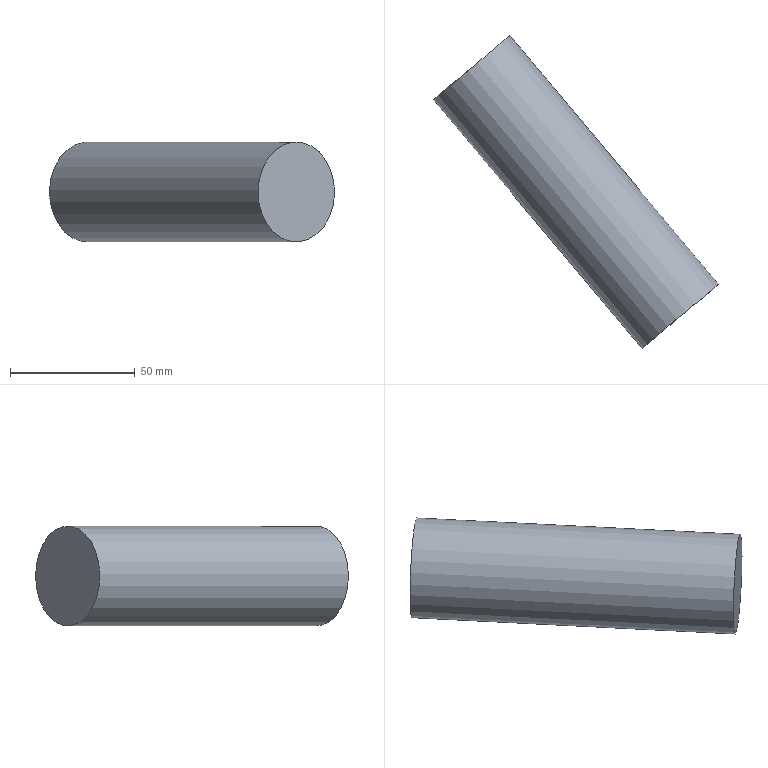Part | NX | features solid 2 | 1 solid | 3 faces | box 114.204 x 125.297 x 40 mm | volume 163363 mm3 | plane 2 | cylinder 1 | commonest cylinder face diameters 40 x1
STEP:
#1=CARTESIAN_POINT('',(828.899,303.057,-194.158));
#2=VERTEX_POINT('',#1);
#3=CARTESIAN_POINT('',(843.885,315.632,-190.));
#4=DIRECTION('',(-0.6428,0.766,0.));
#5=DIRECTION('',(-0.7493,-0.6287,-0.2079));
#6=AXIS2_PLACEMENT_3D('',#3,#4,#5);
#7=CIRCLE('',#6,20.);
#8=EDGE_CURVE('',#2,#2,#7,.F.);
#9=ORIENTED_EDGE('',*,*,#8,.T.);
#10=EDGE_LOOP('',(#9));
#11=FACE_BOUND('',#10,.T.);
#12=CARTESIAN_POINT('',(862.618,331.35,-184.802));
#13=DIRECTION('',(-0.6428,0.766,0.));
#14=DIRECTION('',(0.1593,0.1336,-0.9781));
#15=AXIS2_PLACEMENT_3D('',#12,#13,#14);
#16=PLANE('',#15);
#17=ADVANCED_FACE('',(#11),#16,.F.);
#18=CARTESIAN_POINT('',(745.337,402.643,-194.158));
#19=VERTEX_POINT('',#18);
#20=CARTESIAN_POINT('',(760.323,415.217,-190.));
#21=DIRECTION('',(-0.6428,0.766,0.));
#22=DIRECTION('',(-0.7493,-0.6287,-0.2079));
#23=AXIS2_PLACEMENT_3D('',#20,#21,#22);
#24=CIRCLE('',#23,20.);
#25=EDGE_CURVE('',#19,#19,#24,.F.);
#26=ORIENTED_EDGE('',*,*,#25,.T.);
#27=EDGE_LOOP('',(#26));
#28=FACE_BOUND('',#27,.T.);
#29=ORIENTED_EDGE('',*,*,#8,.F.);
#30=EDGE_LOOP('',(#29));
#31=FACE_BOUND('',#30,.T.);
#32=CARTESIAN_POINT('',(525.705,694.824,-190.));
#33=DIRECTION('',(0.6428,-0.766,0.));
#34=DIRECTION('',(-0.1593,-0.1336,0.9781));
#35=AXIS2_PLACEMENT_3D('',#32,#33,#34);
#36=CYLINDRICAL_SURFACE('',#35,20.);
#37=ADVANCED_FACE('',(#28,#31),#36,.T.);
#38=ORIENTED_EDGE('',*,*,#25,.F.);
#39=EDGE_LOOP('',(#38));
#40=FACE_BOUND('',#39,.T.);
#41=CARTESIAN_POINT('',(782.802,434.08,-183.763));
#42=DIRECTION('',(-0.6428,0.766,0.));
#43=DIRECTION('',(0.1593,0.1336,-0.9781));
#44=AXIS2_PLACEMENT_3D('',#41,#42,#43);
#45=PLANE('',#44);
#46=ADVANCED_FACE('',(#40),#45,.T.);
#47=CLOSED_SHELL('',(#17,#37,#46));
#48=MANIFOLD_SOLID_BREP('',#47);
#49=(LENGTH_UNIT()NAMED_UNIT(*)SI_UNIT(.MILLI.,.METRE.));
#50=UNCERTAINTY_MEASURE_WITH_UNIT(LENGTH_MEASURE(0.00001),#49,'','');
#51=(NAMED_UNIT(*)PLANE_ANGLE_UNIT()SI_UNIT($,.RADIAN.));
#52=(NAMED_UNIT(*)SI_UNIT($,.STERADIAN.)SOLID_ANGLE_UNIT());
#53=(GEOMETRIC_REPRESENTATION_CONTEXT(3)GLOBAL_UNCERTAINTY_ASSIGNED_CONTEXT((#50))GLOBAL_UNIT_ASSIGNED_CONTEXT((#49,#51,#52))REPRESENTATION_CONTEXT('',''));
#54=ADVANCED_BREP_SHAPE_REPRESENTATION('',(#48),#53);